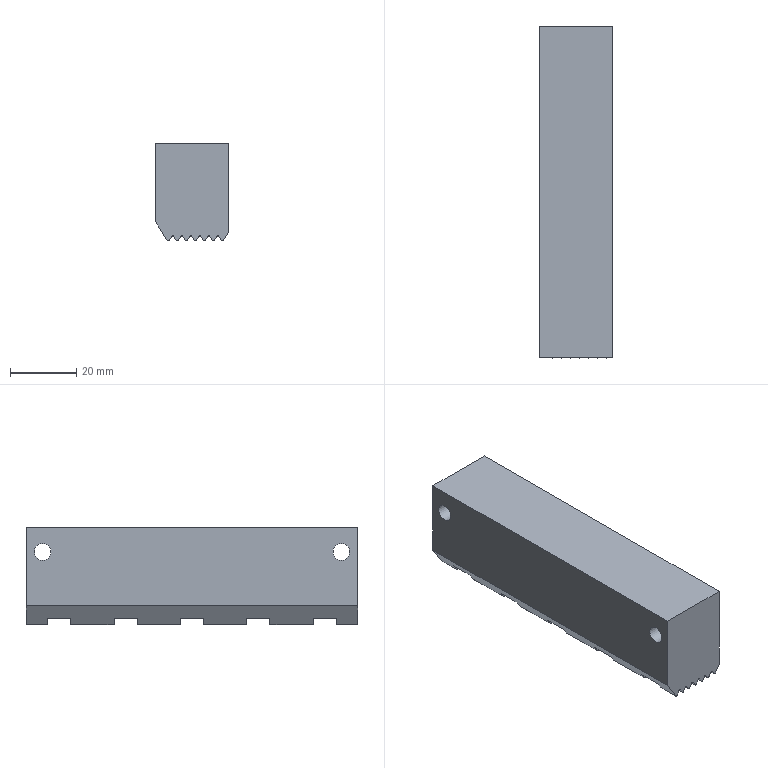Part | STEP file | 1 solid | 174 faces | box 22 x 100 x 29.5 mm | volume 60684 mm3 | plane 94 | cylinder 80 | commonest cylinder face diameters 0.68 x42 0.72 x36 5.02 x2